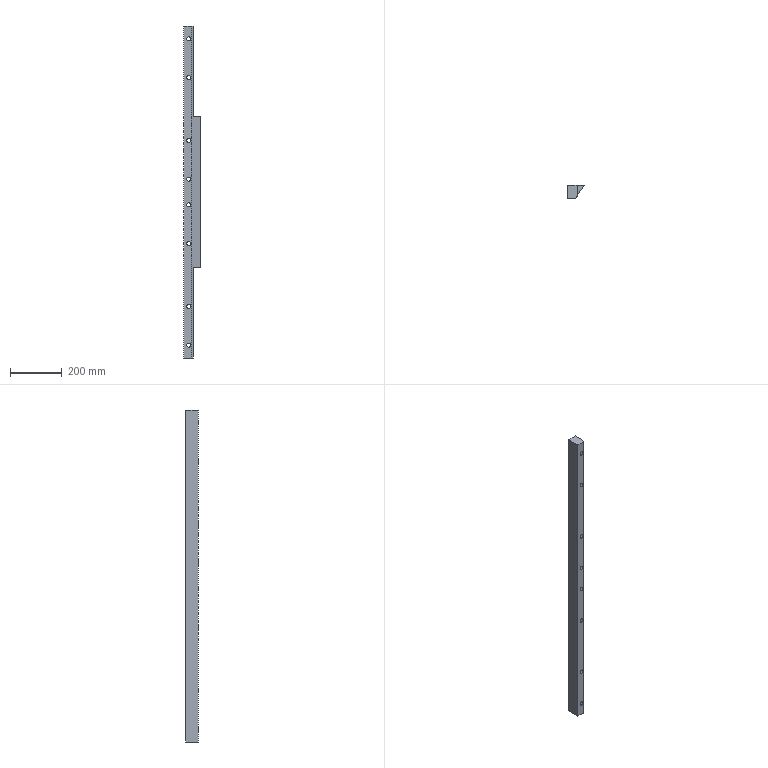Part | SolidWorks | features ICE 3, Extrusion 1, MirrorPattern 1 | 1 solid | 50 faces | box 64 x 50 x 1288 mm | volume 2493147 mm3 | cylinder 32 | plane 18 | commonest cylinder face diameters 16 x16 26 x16
STEP:
#1=CARTESIAN_POINT('',(20.,39.,1225.));
#2=VERTEX_POINT('',#1);
#3=CARTESIAN_POINT('',(20.,39.,1251.));
#4=VERTEX_POINT('',#3);
#5=CARTESIAN_POINT('',(20.,39.,1238.));
#6=DIRECTION('',(0.,1.,0.));
#7=DIRECTION('',(0.,0.,1.));
#8=AXIS2_PLACEMENT_3D('',#5,#6,#7);
#9=CIRCLE('',#8,13.);
#10=EDGE_CURVE('',#2,#4,#9,.T.);
#11=ORIENTED_EDGE('',*,*,#10,.F.);
#12=CARTESIAN_POINT('',(20.,50.,1225.));
#13=VERTEX_POINT('',#12);
#14=CARTESIAN_POINT('',(20.,39.,1225.));
#15=DIRECTION('',(0.,1.,0.));
#16=VECTOR('',#15,1000.);
#17=LINE('',#14,#16);
#18=EDGE_CURVE('',#2,#13,#17,.T.);
#19=ORIENTED_EDGE('',*,*,#18,.T.);
#20=CARTESIAN_POINT('',(20.,50.,1251.));
#21=VERTEX_POINT('',#20);
#22=CARTESIAN_POINT('',(20.,50.,1238.));
#23=DIRECTION('',(0.,1.,0.));
#24=DIRECTION('',(0.,0.,1.));
#25=AXIS2_PLACEMENT_3D('',#22,#23,#24);
#26=CIRCLE('',#25,13.);
#27=EDGE_CURVE('',#13,#21,#26,.T.);
#28=ORIENTED_EDGE('',*,*,#27,.T.);
#29=CARTESIAN_POINT('',(20.,39.,1251.));
#30=DIRECTION('',(0.,1.,0.));
#31=VECTOR('',#30,1000.);
#32=LINE('',#29,#31);
#33=EDGE_CURVE('',#4,#21,#32,.T.);
#34=ORIENTED_EDGE('',*,*,#33,.F.);
#35=EDGE_LOOP('',(#11,#19,#28,#34));
#36=FACE_OUTER_BOUND('',#35,.T.);
#37=CARTESIAN_POINT('',(20.,39.,1238.));
#38=DIRECTION('',(0.,1.,0.));
#39=DIRECTION('',(0.,0.,1.));
#40=AXIS2_PLACEMENT_3D('',#37,#38,#39);
#41=CYLINDRICAL_SURFACE('',#40,13.);
#42=ADVANCED_FACE('',(#36),#41,.F.);
#43=CARTESIAN_POINT('',(20.,39.,1075.));
#44=VERTEX_POINT('',#43);
#45=CARTESIAN_POINT('',(20.,39.,1101.));
#46=VERTEX_POINT('',#45);
#47=CARTESIAN_POINT('',(20.,39.,1088.));
#48=DIRECTION('',(0.,1.,0.));
#49=DIRECTION('',(0.,0.,1.));
#50=AXIS2_PLACEMENT_3D('',#47,#48,#49);
#51=CIRCLE('',#50,13.);
#52=EDGE_CURVE('',#44,#46,#51,.T.);
#53=ORIENTED_EDGE('',*,*,#52,.F.);
#54=CARTESIAN_POINT('',(20.,50.,1075.));
#55=VERTEX_POINT('',#54);
#56=CARTESIAN_POINT('',(20.,39.,1075.));
#57=DIRECTION('',(0.,1.,0.));
#58=VECTOR('',#57,1000.);
#59=LINE('',#56,#58);
#60=EDGE_CURVE('',#44,#55,#59,.T.);
#61=ORIENTED_EDGE('',*,*,#60,.T.);
#62=CARTESIAN_POINT('',(20.,50.,1101.));
#63=VERTEX_POINT('',#62);
#64=CARTESIAN_POINT('',(20.,50.,1088.));
#65=DIRECTION('',(0.,1.,0.));
#66=DIRECTION('',(0.,0.,1.));
#67=AXIS2_PLACEMENT_3D('',#64,#65,#66);
#68=CIRCLE('',#67,13.);
#69=EDGE_CURVE('',#55,#63,#68,.T.);
#70=ORIENTED_EDGE('',*,*,#69,.T.);
#71=CARTESIAN_POINT('',(20.,39.,1101.));
#72=DIRECTION('',(0.,1.,0.));
#73=VECTOR('',#72,1000.);
#74=LINE('',#71,#73);
#75=EDGE_CURVE('',#46,#63,#74,.T.);
#76=ORIENTED_EDGE('',*,*,#75,.F.);
#77=EDGE_LOOP('',(#53,#61,#70,#76));
#78=FACE_OUTER_BOUND('',#77,.T.);
#79=CARTESIAN_POINT('',(20.,39.,1088.));
#80=DIRECTION('',(0.,1.,0.));
#81=DIRECTION('',(0.,0.,1.));
#82=AXIS2_PLACEMENT_3D('',#79,#80,#81);
#83=CYLINDRICAL_SURFACE('',#82,13.);
#84=ADVANCED_FACE('',(#78),#83,.F.);
#85=CARTESIAN_POINT('',(20.,39.,831.));
#86=VERTEX_POINT('',#85);
#87=CARTESIAN_POINT('',(20.,39.,857.));
#88=VERTEX_POINT('',#87);
#89=CARTESIAN_POINT('',(20.,39.,844.));
#90=DIRECTION('',(0.,1.,0.));
#91=DIRECTION('',(0.,0.,1.));
#92=AXIS2_PLACEMENT_3D('',#89,#90,#91);
#93=CIRCLE('',#92,13.);
#94=EDGE_CURVE('',#86,#88,#93,.T.);
#95=ORIENTED_EDGE('',*,*,#94,.F.);
#96=CARTESIAN_POINT('',(20.,50.,831.));
#97=VERTEX_POINT('',#96);
#98=CARTESIAN_POINT('',(20.,39.,831.));
#99=DIRECTION('',(0.,1.,0.));
#100=VECTOR('',#99,1000.);
#101=LINE('',#98,#100);
#102=EDGE_CURVE('',#86,#97,#101,.T.);
#103=ORIENTED_EDGE('',*,*,#102,.T.);
#104=CARTESIAN_POINT('',(20.,50.,857.));
#105=VERTEX_POINT('',#104);
#106=CARTESIAN_POINT('',(20.,50.,844.));
#107=DIRECTION('',(0.,1.,0.));
#108=DIRECTION('',(0.,0.,1.));
#109=AXIS2_PLACEMENT_3D('',#106,#107,#108);
#110=CIRCLE('',#109,13.);
#111=EDGE_CURVE('',#97,#105,#110,.T.);
#112=ORIENTED_EDGE('',*,*,#111,.T.);
#113=CARTESIAN_POINT('',(20.,39.,857.));
#114=DIRECTION('',(0.,1.,0.));
#115=VECTOR('',#114,1000.);
#116=LINE('',#113,#115);
#117=EDGE_CURVE('',#88,#105,#116,.T.);
#118=ORIENTED_EDGE('',*,*,#117,.F.);
#119=EDGE_LOOP('',(#95,#103,#112,#118));
#120=FACE_OUTER_BOUND('',#119,.T.);
#121=CARTESIAN_POINT('',(20.,39.,844.));
#122=DIRECTION('',(0.,1.,0.));
#123=DIRECTION('',(0.,0.,1.));
#124=AXIS2_PLACEMENT_3D('',#121,#122,#123);
#125=CYLINDRICAL_SURFACE('',#124,13.);
#126=ADVANCED_FACE('',(#120),#125,.F.);
#127=CARTESIAN_POINT('',(20.,39.,681.));
#128=VERTEX_POINT('',#127);
#129=CARTESIAN_POINT('',(20.,39.,707.));
#130=VERTEX_POINT('',#129);
#131=CARTESIAN_POINT('',(20.,39.,694.));
#132=DIRECTION('',(0.,1.,0.));
#133=DIRECTION('',(0.,0.,1.));
#134=AXIS2_PLACEMENT_3D('',#131,#132,#133);
#135=CIRCLE('',#134,13.);
#136=EDGE_CURVE('',#128,#130,#135,.T.);
#137=ORIENTED_EDGE('',*,*,#136,.F.);
#138=CARTESIAN_POINT('',(20.,50.,681.));
#139=VERTEX_POINT('',#138);
#140=CARTESIAN_POINT('',(20.,39.,681.));
#141=DIRECTION('',(0.,1.,0.));
#142=VECTOR('',#141,1000.);
#143=LINE('',#140,#142);
#144=EDGE_CURVE('',#128,#139,#143,.T.);
#145=ORIENTED_EDGE('',*,*,#144,.T.);
#146=CARTESIAN_POINT('',(20.,50.,707.));
#147=VERTEX_POINT('',#146);
#148=CARTESIAN_POINT('',(20.,50.,694.));
#149=DIRECTION('',(0.,1.,0.));
#150=DIRECTION('',(0.,0.,1.));
#151=AXIS2_PLACEMENT_3D('',#148,#149,#150);
#152=CIRCLE('',#151,13.);
#153=EDGE_CURVE('',#139,#147,#152,.T.);
#154=ORIENTED_EDGE('',*,*,#153,.T.);
#155=CARTESIAN_POINT('',(20.,39.,707.));
#156=DIRECTION('',(0.,1.,0.));
#157=VECTOR('',#156,1000.);
#158=LINE('',#155,#157);
#159=EDGE_CURVE('',#130,#147,#158,.T.);
#160=ORIENTED_EDGE('',*,*,#159,.F.);
#161=EDGE_LOOP('',(#137,#145,#154,#160));
#162=FACE_OUTER_BOUND('',#161,.T.);
#163=CARTESIAN_POINT('',(20.,39.,694.));
#164=DIRECTION('',(0.,1.,0.));
#165=DIRECTION('',(0.,0.,1.));
#166=AXIS2_PLACEMENT_3D('',#163,#164,#165);
#167=CYLINDRICAL_SURFACE('',#166,13.);
#168=ADVANCED_FACE('',(#162),#167,.F.);
#169=CARTESIAN_POINT('',(20.,39.,581.));
#170=VERTEX_POINT('',#169);
#171=CARTESIAN_POINT('',(20.,39.,607.));
#172=VERTEX_POINT('',#171);
#173=CARTESIAN_POINT('',(20.,39.,594.));
#174=DIRECTION('',(0.,1.,0.));
#175=DIRECTION('',(0.,0.,1.));
#176=AXIS2_PLACEMENT_3D('',#173,#174,#175);
#177=CIRCLE('',#176,13.);
#178=EDGE_CURVE('',#170,#172,#177,.T.);
#179=ORIENTED_EDGE('',*,*,#178,.F.);
#180=CARTESIAN_POINT('',(20.,50.,581.));
#181=VERTEX_POINT('',#180);
#182=CARTESIAN_POINT('',(20.,39.,581.));
#183=DIRECTION('',(0.,1.,0.));
#184=VECTOR('',#183,1000.);
#185=LINE('',#182,#184);
#186=EDGE_CURVE('',#170,#181,#185,.T.);
#187=ORIENTED_EDGE('',*,*,#186,.T.);
#188=CARTESIAN_POINT('',(20.,50.,607.));
#189=VERTEX_POINT('',#188);
#190=CARTESIAN_POINT('',(20.,50.,594.));
#191=DIRECTION('',(0.,1.,0.));
#192=DIRECTION('',(0.,0.,1.));
#193=AXIS2_PLACEMENT_3D('',#190,#191,#192);
#194=CIRCLE('',#193,13.);
#195=EDGE_CURVE('',#181,#189,#194,.T.);
#196=ORIENTED_EDGE('',*,*,#195,.T.);
#197=CARTESIAN_POINT('',(20.,39.,607.));
#198=DIRECTION('',(0.,1.,0.));
#199=VECTOR('',#198,1000.);
#200=LINE('',#197,#199);
#201=EDGE_CURVE('',#172,#189,#200,.T.);
#202=ORIENTED_EDGE('',*,*,#201,.F.);
#203=EDGE_LOOP('',(#179,#187,#196,#202));
#204=FACE_OUTER_BOUND('',#203,.T.);
#205=CARTESIAN_POINT('',(20.,39.,594.));
#206=DIRECTION('',(0.,1.,0.));
#207=DIRECTION('',(0.,0.,1.));
#208=AXIS2_PLACEMENT_3D('',#205,#206,#207);
#209=CYLINDRICAL_SURFACE('',#208,13.);
#210=ADVANCED_FACE('',(#204),#209,.F.);
#211=CARTESIAN_POINT('',(20.,39.,431.));
#212=VERTEX_POINT('',#211);
#213=CARTESIAN_POINT('',(20.,39.,457.));
#214=VERTEX_POINT('',#213);
#215=CARTESIAN_POINT('',(20.,39.,444.));
#216=DIRECTION('',(0.,1.,0.));
#217=DIRECTION('',(0.,0.,1.));
#218=AXIS2_PLACEMENT_3D('',#215,#216,#217);
#219=CIRCLE('',#218,13.);
#220=EDGE_CURVE('',#212,#214,#219,.T.);
#221=ORIENTED_EDGE('',*,*,#220,.F.);
#222=CARTESIAN_POINT('',(20.,50.,431.));
#223=VERTEX_POINT('',#222);
#224=CARTESIAN_POINT('',(20.,39.,431.));
#225=DIRECTION('',(0.,1.,0.));
#226=VECTOR('',#225,1000.);
#227=LINE('',#224,#226);
#228=EDGE_CURVE('',#212,#223,#227,.T.);
#229=ORIENTED_EDGE('',*,*,#228,.T.);
#230=CARTESIAN_POINT('',(20.,50.,457.));
#231=VERTEX_POINT('',#230);
#232=CARTESIAN_POINT('',(20.,50.,444.));
#233=DIRECTION('',(0.,1.,0.));
#234=DIRECTION('',(0.,0.,1.));
#235=AXIS2_PLACEMENT_3D('',#232,#233,#234);
#236=CIRCLE('',#235,13.);
#237=EDGE_CURVE('',#223,#231,#236,.T.);
#238=ORIENTED_EDGE('',*,*,#237,.T.);
#239=CARTESIAN_POINT('',(20.,39.,457.));
#240=DIRECTION('',(0.,1.,0.));
#241=VECTOR('',#240,1000.);
#242=LINE('',#239,#241);
#243=EDGE_CURVE('',#214,#231,#242,.T.);
#244=ORIENTED_EDGE('',*,*,#243,.F.);
#245=EDGE_LOOP('',(#221,#229,#238,#244));
#246=FACE_OUTER_BOUND('',#245,.T.);
#247=CARTESIAN_POINT('',(20.,39.,444.));
#248=DIRECTION('',(0.,1.,0.));
#249=DIRECTION('',(0.,0.,1.));
#250=AXIS2_PLACEMENT_3D('',#247,#248,#249);
#251=CYLINDRICAL_SURFACE('',#250,13.);
#252=ADVANCED_FACE('',(#246),#251,.F.);
#253=CARTESIAN_POINT('',(20.,39.,187.));
#254=VERTEX_POINT('',#253);
#255=CARTESIAN_POINT('',(20.,39.,213.));
#256=VERTEX_POINT('',#255);
#257=CARTESIAN_POINT('',(20.,39.,200.));
#258=DIRECTION('',(0.,1.,0.));
#259=DIRECTION('',(0.,0.,1.));
#260=AXIS2_PLACEMENT_3D('',#257,#258,#259);
#261=CIRCLE('',#260,13.);
#262=EDGE_CURVE('',#254,#256,#261,.T.);
#263=ORIENTED_EDGE('',*,*,#262,.F.);
#264=CARTESIAN_POINT('',(20.,50.,187.));
#265=VERTEX_POINT('',#264);
#266=CARTESIAN_POINT('',(20.,39.,187.));
#267=DIRECTION('',(0.,1.,0.));
#268=VECTOR('',#267,1000.);
#269=LINE('',#266,#268);
#270=EDGE_CURVE('',#254,#265,#269,.T.);
#271=ORIENTED_EDGE('',*,*,#270,.T.);
#272=CARTESIAN_POINT('',(20.,50.,213.));
#273=VERTEX_POINT('',#272);
#274=CARTESIAN_POINT('',(20.,50.,200.));
#275=DIRECTION('',(0.,1.,0.));
#276=DIRECTION('',(0.,0.,1.));
#277=AXIS2_PLACEMENT_3D('',#274,#275,#276);
#278=CIRCLE('',#277,13.);
#279=EDGE_CURVE('',#265,#273,#278,.T.);
#280=ORIENTED_EDGE('',*,*,#279,.T.);
#281=CARTESIAN_POINT('',(20.,39.,213.));
#282=DIRECTION('',(0.,1.,0.));
#283=VECTOR('',#282,1000.);
#284=LINE('',#281,#283);
#285=EDGE_CURVE('',#256,#273,#284,.T.);
#286=ORIENTED_EDGE('',*,*,#285,.F.);
#287=EDGE_LOOP('',(#263,#271,#280,#286));
#288=FACE_OUTER_BOUND('',#287,.T.);
#289=CARTESIAN_POINT('',(20.,39.,200.));
#290=DIRECTION('',(0.,1.,0.));
#291=DIRECTION('',(0.,0.,1.));
#292=AXIS2_PLACEMENT_3D('',#289,#290,#291);
#293=CYLINDRICAL_SURFACE('',#292,13.);
#294=ADVANCED_FACE('',(#288),#293,.F.);
#295=CARTESIAN_POINT('',(20.,39.,37.));
#296=VERTEX_POINT('',#295);
#297=CARTESIAN_POINT('',(20.,39.,63.));
#298=VERTEX_POINT('',#297);
#299=CARTESIAN_POINT('',(20.,39.,50.));
#300=DIRECTION('',(0.,1.,0.));
#301=DIRECTION('',(0.,0.,1.));
#302=AXIS2_PLACEMENT_3D('',#299,#300,#301);
#303=CIRCLE('',#302,13.);
#304=EDGE_CURVE('',#296,#298,#303,.T.);
#305=ORIENTED_EDGE('',*,*,#304,.F.);
#306=CARTESIAN_POINT('',(20.,50.,37.));
#307=VERTEX_POINT('',#306);
#308=CARTESIAN_POINT('',(20.,39.,37.));
#309=DIRECTION('',(0.,1.,0.));
#310=VECTOR('',#309,1000.);
#311=LINE('',#308,#310);
#312=EDGE_CURVE('',#296,#307,#311,.T.);
#313=ORIENTED_EDGE('',*,*,#312,.T.);
#314=CARTESIAN_POINT('',(20.,50.,63.));
#315=VERTEX_POINT('',#314);
#316=CARTESIAN_POINT('',(20.,50.,50.));
#317=DIRECTION('',(0.,1.,0.));
#318=DIRECTION('',(0.,0.,1.));
#319=AXIS2_PLACEMENT_3D('',#316,#317,#318);
#320=CIRCLE('',#319,13.);
#321=EDGE_CURVE('',#307,#315,#320,.T.);
#322=ORIENTED_EDGE('',*,*,#321,.T.);
#323=CARTESIAN_POINT('',(20.,39.,63.));
#324=DIRECTION('',(0.,1.,0.));
#325=VECTOR('',#324,1000.);
#326=LINE('',#323,#325);
#327=EDGE_CURVE('',#298,#315,#326,.T.);
#328=ORIENTED_EDGE('',*,*,#327,.F.);
#329=EDGE_LOOP('',(#305,#313,#322,#328));
#330=FACE_OUTER_BOUND('',#329,.T.);
#331=CARTESIAN_POINT('',(20.,39.,50.));
#332=DIRECTION('',(0.,1.,0.));
#333=DIRECTION('',(0.,0.,1.));
#334=AXIS2_PLACEMENT_3D('',#331,#332,#333);
#335=CYLINDRICAL_SURFACE('',#334,13.);
#336=ADVANCED_FACE('',(#330),#335,.F.);
#337=CARTESIAN_POINT('',(20.,0.,42.));
#338=VERTEX_POINT('',#337);
#339=CARTESIAN_POINT('',(20.,0.,58.));
#340=VERTEX_POINT('',#339);
#341=CARTESIAN_POINT('',(20.,0.,50.));
#342=DIRECTION('',(0.,1.,0.));
#343=DIRECTION('',(0.,0.,1.));
#344=AXIS2_PLACEMENT_3D('',#341,#342,#343);
#345=CIRCLE('',#344,8.);
#346=EDGE_CURVE('',#338,#340,#345,.T.);
#347=ORIENTED_EDGE('',*,*,#346,.F.);
#348=CARTESIAN_POINT('',(20.,39.,42.));
#349=VERTEX_POINT('',#348);
#350=CARTESIAN_POINT('',(20.,-675.,42.));
#351=DIRECTION('',(0.,1.,0.));
#352=VECTOR('',#351,1000.);
#353=LINE('',#350,#352);
#354=EDGE_CURVE('',#338,#349,#353,.T.);
#355=ORIENTED_EDGE('',*,*,#354,.T.);
#356=CARTESIAN_POINT('',(20.,39.,58.));
#357=VERTEX_POINT('',#356);
#358=CARTESIAN_POINT('',(20.,39.,50.));
#359=DIRECTION('',(0.,-1.,0.));
#360=DIRECTION('',(0.,0.,1.));
#361=AXIS2_PLACEMENT_3D('',#358,#359,#360);
#362=CIRCLE('',#361,8.);
#363=EDGE_CURVE('',#357,#349,#362,.T.);
#364=ORIENTED_EDGE('',*,*,#363,.F.);
#365=CARTESIAN_POINT('',(20.,-675.,58.));
#366=DIRECTION('',(0.,1.,0.));
#367=VECTOR('',#366,1000.);
#368=LINE('',#365,#367);
#369=EDGE_CURVE('',#340,#357,#368,.T.);
#370=ORIENTED_EDGE('',*,*,#369,.F.);
#371=EDGE_LOOP('',(#347,#355,#364,#370));
#372=FACE_OUTER_BOUND('',#371,.T.);
#373=CARTESIAN_POINT('',(20.,-675.,50.));
#374=DIRECTION('',(0.,1.,0.));
#375=DIRECTION('',(0.,0.,1.));
#376=AXIS2_PLACEMENT_3D('',#373,#374,#375);
#377=CYLINDRICAL_SURFACE('',#376,8.);
#378=ADVANCED_FACE('',(#372),#377,.F.);
#379=CARTESIAN_POINT('',(20.,0.,192.));
#380=VERTEX_POINT('',#379);
#381=CARTESIAN_POINT('',(20.,0.,208.));
#382=VERTEX_POINT('',#381);
#383=CARTESIAN_POINT('',(20.,0.,200.));
#384=DIRECTION('',(0.,1.,0.));
#385=DIRECTION('',(0.,0.,1.));
#386=AXIS2_PLACEMENT_3D('',#383,#384,#385);
#387=CIRCLE('',#386,8.);
#388=EDGE_CURVE('',#380,#382,#387,.T.);
#389=ORIENTED_EDGE('',*,*,#388,.F.);
#390=CARTESIAN_POINT('',(20.,39.,192.));
#391=VERTEX_POINT('',#390);
#392=CARTESIAN_POINT('',(20.,-675.,192.));
#393=DIRECTION('',(0.,1.,0.));
#394=VECTOR('',#393,1000.);
#395=LINE('',#392,#394);
#396=EDGE_CURVE('',#380,#391,#395,.T.);
#397=ORIENTED_EDGE('',*,*,#396,.T.);
#398=CARTESIAN_POINT('',(20.,39.,208.));
#399=VERTEX_POINT('',#398);
#400=CARTESIAN_POINT('',(20.,39.,200.));
#401=DIRECTION('',(0.,-1.,0.));
#402=DIRECTION('',(0.,0.,1.));
#403=AXIS2_PLACEMENT_3D('',#400,#401,#402);
#404=CIRCLE('',#403,8.);
#405=EDGE_CURVE('',#399,#391,#404,.T.);
#406=ORIENTED_EDGE('',*,*,#405,.F.);
#407=CARTESIAN_POINT('',(20.,-675.,208.));
#408=DIRECTION('',(0.,1.,0.));
#409=VECTOR('',#408,1000.);
#410=LINE('',#407,#409);
#411=EDGE_CURVE('',#382,#399,#410,.T.);
#412=ORIENTED_EDGE('',*,*,#411,.F.);
#413=EDGE_LOOP('',(#389,#397,#406,#412));
#414=FACE_OUTER_BOUND('',#413,.T.);
#415=CARTESIAN_POINT('',(20.,-675.,200.));
#416=DIRECTION('',(0.,1.,0.));
#417=DIRECTION('',(0.,0.,1.));
#418=AXIS2_PLACEMENT_3D('',#415,#416,#417);
#419=CYLINDRICAL_SURFACE('',#418,8.);
#420=ADVANCED_FACE('',(#414),#419,.F.);
#421=CARTESIAN_POINT('',(20.,0.,436.));
#422=VERTEX_POINT('',#421);
#423=CARTESIAN_POINT('',(20.,0.,452.));
#424=VERTEX_POINT('',#423);
#425=CARTESIAN_POINT('',(20.,0.,444.));
#426=DIRECTION('',(0.,1.,0.));
#427=DIRECTION('',(0.,0.,1.));
#428=AXIS2_PLACEMENT_3D('',#425,#426,#427);
#429=CIRCLE('',#428,8.);
#430=EDGE_CURVE('',#422,#424,#429,.T.);
#431=ORIENTED_EDGE('',*,*,#430,.F.);
#432=CARTESIAN_POINT('',(20.,39.,436.));
#433=VERTEX_POINT('',#432);
#434=CARTESIAN_POINT('',(20.,-675.,436.));
#435=DIRECTION('',(0.,1.,0.));
#436=VECTOR('',#435,1000.);
#437=LINE('',#434,#436);
#438=EDGE_CURVE('',#422,#433,#437,.T.);
#439=ORIENTED_EDGE('',*,*,#438,.T.);
#440=CARTESIAN_POINT('',(20.,39.,452.));
#441=VERTEX_POINT('',#440);
#442=CARTESIAN_POINT('',(20.,39.,444.));
#443=DIRECTION('',(0.,-1.,0.));
#444=DIRECTION('',(0.,0.,1.));
#445=AXIS2_PLACEMENT_3D('',#442,#443,#444);
#446=CIRCLE('',#445,8.);
#447=EDGE_CURVE('',#441,#433,#446,.T.);
#448=ORIENTED_EDGE('',*,*,#447,.F.);
#449=CARTESIAN_POINT('',(20.,-675.,452.));
#450=DIRECTION('',(0.,1.,0.));
#451=VECTOR('',#450,1000.);
#452=LINE('',#449,#451);
#453=EDGE_CURVE('',#424,#441,#452,.T.);
#454=ORIENTED_EDGE('',*,*,#453,.F.);
#455=EDGE_LOOP('',(#431,#439,#448,#454));
#456=FACE_OUTER_BOUND('',#455,.T.);
#457=CARTESIAN_POINT('',(20.,-675.,444.));
#458=DIRECTION('',(0.,1.,0.));
#459=DIRECTION('',(0.,0.,1.));
#460=AXIS2_PLACEMENT_3D('',#457,#458,#459);
#461=CYLINDRICAL_SURFACE('',#460,8.);
#462=ADVANCED_FACE('',(#456),#461,.F.);
#463=CARTESIAN_POINT('',(20.,0.,586.));
#464=VERTEX_POINT('',#463);
#465=CARTESIAN_POINT('',(20.,0.,602.));
#466=VERTEX_POINT('',#465);
#467=CARTESIAN_POINT('',(20.,0.,594.));
#468=DIRECTION('',(0.,1.,0.));
#469=DIRECTION('',(0.,0.,1.));
#470=AXIS2_PLACEMENT_3D('',#467,#468,#469);
#471=CIRCLE('',#470,8.);
#472=EDGE_CURVE('',#464,#466,#471,.T.);
#473=ORIENTED_EDGE('',*,*,#472,.F.);
#474=CARTESIAN_POINT('',(20.,39.,586.));
#475=VERTEX_POINT('',#474);
#476=CARTESIAN_POINT('',(20.,-675.,586.));
#477=DIRECTION('',(0.,1.,0.));
#478=VECTOR('',#477,1000.);
#479=LINE('',#476,#478);
#480=EDGE_CURVE('',#464,#475,#479,.T.);
#481=ORIENTED_EDGE('',*,*,#480,.T.);
#482=CARTESIAN_POINT('',(20.,39.,602.));
#483=VERTEX_POINT('',#482);
#484=CARTESIAN_POINT('',(20.,39.,594.));
#485=DIRECTION('',(0.,-1.,0.));
#486=DIRECTION('',(0.,0.,1.));
#487=AXIS2_PLACEMENT_3D('',#484,#485,#486);
#488=CIRCLE('',#487,8.);
#489=EDGE_CURVE('',#483,#475,#488,.T.);
#490=ORIENTED_EDGE('',*,*,#489,.F.);
#491=CARTESIAN_POINT('',(20.,-675.,602.));
#492=DIRECTION('',(0.,1.,0.));
#493=VECTOR('',#492,1000.);
#494=LINE('',#491,#493);
#495=EDGE_CURVE('',#466,#483,#494,.T.);
#496=ORIENTED_EDGE('',*,*,#495,.F.);
#497=EDGE_LOOP('',(#473,#481,#490,#496));
#498=FACE_OUTER_BOUND('',#497,.T.);
#499=CARTESIAN_POINT('',(20.,-675.,594.));
#500=DIRECTION('',(0.,1.,0.));
#501=DIRECTION('',(0.,0.,1.));
#502=AXIS2_PLACEMENT_3D('',#499,#500,#501);
#503=CYLINDRICAL_SURFACE('',#502,8.);
#504=ADVANCED_FACE('',(#498),#503,.F.);
#505=CARTESIAN_POINT('',(20.,0.,686.));
#506=VERTEX_POINT('',#505);
#507=CARTESIAN_POINT('',(20.,0.,702.));
#508=VERTEX_POINT('',#507);
#509=CARTESIAN_POINT('',(20.,0.,694.));
#510=DIRECTION('',(0.,1.,0.));
#511=DIRECTION('',(0.,0.,1.));
#512=AXIS2_PLACEMENT_3D('',#509,#510,#511);
#513=CIRCLE('',#512,8.);
#514=EDGE_CURVE('',#506,#508,#513,.T.);
#515=ORIENTED_EDGE('',*,*,#514,.F.);
#516=CARTESIAN_POINT('',(20.,39.,686.));
#517=VERTEX_POINT('',#516);
#518=CARTESIAN_POINT('',(20.,-675.,686.));
#519=DIRECTION('',(0.,1.,0.));
#520=VECTOR('',#519,1000.);
#521=LINE('',#518,#520);
#522=EDGE_CURVE('',#506,#517,#521,.T.);
#523=ORIENTED_EDGE('',*,*,#522,.T.);
#524=CARTESIAN_POINT('',(20.,39.,702.));
#525=VERTEX_POINT('',#524);
#526=CARTESIAN_POINT('',(20.,39.,694.));
#527=DIRECTION('',(0.,-1.,0.));
#528=DIRECTION('',(0.,0.,1.));
#529=AXIS2_PLACEMENT_3D('',#526,#527,#528);
#530=CIRCLE('',#529,8.);
#531=EDGE_CURVE('',#525,#517,#530,.T.);
#532=ORIENTED_EDGE('',*,*,#531,.F.);
#533=CARTESIAN_POINT('',(20.,-675.,702.));
#534=DIRECTION('',(0.,1.,0.));
#535=VECTOR('',#534,1000.);
#536=LINE('',#533,#535);
#537=EDGE_CURVE('',#508,#525,#536,.T.);
#538=ORIENTED_EDGE('',*,*,#537,.F.);
#539=EDGE_LOOP('',(#515,#523,#532,#538));
#540=FACE_OUTER_BOUND('',#539,.T.);
#541=CARTESIAN_POINT('',(20.,-675.,694.));
#542=DIRECTION('',(0.,1.,0.));
#543=DIRECTION('',(0.,0.,1.));
#544=AXIS2_PLACEMENT_3D('',#541,#542,#543);
#545=CYLINDRICAL_SURFACE('',#544,8.);
#546=ADVANCED_FACE('',(#540),#545,.F.);
#547=CARTESIAN_POINT('',(20.,0.,836.));
#548=VERTEX_POINT('',#547);
#549=CARTESIAN_POINT('',(20.,0.,852.));
#550=VERTEX_POINT('',#549);
#551=CARTESIAN_POINT('',(20.,0.,844.));
#552=DIRECTION('',(0.,1.,0.));
#553=DIRECTION('',(0.,0.,1.));
#554=AXIS2_PLACEMENT_3D('',#551,#552,#553);
#555=CIRCLE('',#554,8.);
#556=EDGE_CURVE('',#548,#550,#555,.T.);
#557=ORIENTED_EDGE('',*,*,#556,.F.);
#558=CARTESIAN_POINT('',(20.,39.,836.));
#559=VERTEX_POINT('',#558);
#560=CARTESIAN_POINT('',(20.,-675.,836.));
#561=DIRECTION('',(0.,1.,0.));
#562=VECTOR('',#561,1000.);
#563=LINE('',#560,#562);
#564=EDGE_CURVE('',#548,#559,#563,.T.);
#565=ORIENTED_EDGE('',*,*,#564,.T.);
#566=CARTESIAN_POINT('',(20.,39.,852.));
#567=VERTEX_POINT('',#566);
#568=CARTESIAN_POINT('',(20.,39.,844.));
#569=DIRECTION('',(0.,-1.,0.));
#570=DIRECTION('',(0.,0.,1.));
#571=AXIS2_PLACEMENT_3D('',#568,#569,#570);
#572=CIRCLE('',#571,8.);
#573=EDGE_CURVE('',#567,#559,#572,.T.);
#574=ORIENTED_EDGE('',*,*,#573,.F.);
#575=CARTESIAN_POINT('',(20.,-675.,852.));
#576=DIRECTION('',(0.,1.,0.));
#577=VECTOR('',#576,1000.);
#578=LINE('',#575,#577);
#579=EDGE_CURVE('',#550,#567,#578,.T.);
#580=ORIENTED_EDGE('',*,*,#579,.F.);
#581=EDGE_LOOP('',(#557,#565,#574,#580));
#582=FACE_OUTER_BOUND('',#581,.T.);
#583=CARTESIAN_POINT('',(20.,-675.,844.));
#584=DIRECTION('',(0.,1.,0.));
#585=DIRECTION('',(0.,0.,1.));
#586=AXIS2_PLACEMENT_3D('',#583,#584,#585);
#587=CYLINDRICAL_SURFACE('',#586,8.);
#588=ADVANCED_FACE('',(#582),#587,.F.);
#589=CARTESIAN_POINT('',(20.,0.,1080.));
#590=VERTEX_POINT('',#589);
#591=CARTESIAN_POINT('',(20.,0.,1096.));
#592=VERTEX_POINT('',#591);
#593=CARTESIAN_POINT('',(20.,0.,1088.));
#594=DIRECTION('',(0.,1.,0.));
#595=DIRECTION('',(0.,0.,1.));
#596=AXIS2_PLACEMENT_3D('',#593,#594,#595);
#597=CIRCLE('',#596,8.);
#598=EDGE_CURVE('',#590,#592,#597,.T.);
#599=ORIENTED_EDGE('',*,*,#598,.F.);
#600=CARTESIAN_POINT('',(20.,39.,1080.));
#601=VERTEX_POINT('',#600);
#602=CARTESIAN_POINT('',(20.,-675.,1080.));
#603=DIRECTION('',(0.,1.,0.));
#604=VECTOR('',#603,1000.);
#605=LINE('',#602,#604);
#606=EDGE_CURVE('',#590,#601,#605,.T.);
#607=ORIENTED_EDGE('',*,*,#606,.T.);
#608=CARTESIAN_POINT('',(20.,39.,1096.));
#609=VERTEX_POINT('',#608);
#610=CARTESIAN_POINT('',(20.,39.,1088.));
#611=DIRECTION('',(0.,-1.,0.));
#612=DIRECTION('',(0.,0.,1.));
#613=AXIS2_PLACEMENT_3D('',#610,#611,#612);
#614=CIRCLE('',#613,8.);
#615=EDGE_CURVE('',#609,#601,#614,.T.);
#616=ORIENTED_EDGE('',*,*,#615,.F.);
#617=CARTESIAN_POINT('',(20.,-675.,1096.));
#618=DIRECTION('',(0.,1.,0.));
#619=VECTOR('',#618,1000.);
#620=LINE('',#617,#619);
#621=EDGE_CURVE('',#592,#609,#620,.T.);
#622=ORIENTED_EDGE('',*,*,#621,.F.);
#623=EDGE_LOOP('',(#599,#607,#616,#622));
#624=FACE_OUTER_BOUND('',#623,.T.);
#625=CARTESIAN_POINT('',(20.,-675.,1088.));
#626=DIRECTION('',(0.,1.,0.));
#627=DIRECTION('',(0.,0.,1.));
#628=AXIS2_PLACEMENT_3D('',#625,#626,#627);
#629=CYLINDRICAL_SURFACE('',#628,8.);
#630=ADVANCED_FACE('',(#624),#629,.F.);
#631=CARTESIAN_POINT('',(20.,0.,1230.));
#632=VERTEX_POINT('',#631);
#633=CARTESIAN_POINT('',(20.,0.,1246.));
#634=VERTEX_POINT('',#633);
#635=CARTESIAN_POINT('',(20.,0.,1238.));
#636=DIRECTION('',(0.,1.,0.));
#637=DIRECTION('',(0.,0.,1.));
#638=AXIS2_PLACEMENT_3D('',#635,#636,#637);
#639=CIRCLE('',#638,8.);
#640=EDGE_CURVE('',#632,#634,#639,.T.);
#641=ORIENTED_EDGE('',*,*,#640,.F.);
#642=CARTESIAN_POINT('',(20.,39.,1230.));
#643=VERTEX_POINT('',#642);
#644=CARTESIAN_POINT('',(20.,-675.,1230.));
#645=DIRECTION('',(0.,1.,0.));
#646=VECTOR('',#645,1000.);
#647=LINE('',#644,#646);
#648=EDGE_CURVE('',#632,#643,#647,.T.);
#649=ORIENTED_EDGE('',*,*,#648,.T.);
#650=CARTESIAN_POINT('',(20.,39.,1246.));
#651=VERTEX_POINT('',#650);
#652=CARTESIAN_POINT('',(20.,39.,1238.));
#653=DIRECTION('',(0.,-1.,0.));
#654=DIRECTION('',(0.,0.,1.));
#655=AXIS2_PLACEMENT_3D('',#652,#653,#654);
#656=CIRCLE('',#655,8.);
#657=EDGE_CURVE('',#651,#643,#656,.T.);
#658=ORIENTED_EDGE('',*,*,#657,.F.);
#659=CARTESIAN_POINT('',(20.,-675.,1246.));
#660=DIRECTION('',(0.,1.,0.));
#661=VECTOR('',#660,1000.);
#662=LINE('',#659,#661);
#663=EDGE_CURVE('',#634,#651,#662,.T.);
#664=ORIENTED_EDGE('',*,*,#663,.F.);
#665=EDGE_LOOP('',(#641,#649,#658,#664));
#666=FACE_OUTER_BOUND('',#665,.T.);
#667=CARTESIAN_POINT('',(20.,-675.,1238.));
#668=DIRECTION('',(0.,1.,0.));
#669=DIRECTION('',(0.,0.,1.));
#670=AXIS2_PLACEMENT_3D('',#667,#668,#669);
#671=CYLINDRICAL_SURFACE('',#670,8.);
#672=ADVANCED_FACE('',(#666),#671,.F.);
#673=CARTESIAN_POINT('',(36.,10.,350.));
#674=VERTEX_POINT('',#673);
#675=CARTESIAN_POINT('',(36.,10.,0.));
#676=VERTEX_POINT('',#675);
#677=CARTESIAN_POINT('',(36.,10.,350.));
#678=DIRECTION('',(0.,0.,-1.));
#679=VECTOR('',#678,1000.);
#680=LINE('',#677,#679);
#681=EDGE_CURVE('',#674,#676,#680,.T.);
#682=ORIENTED_EDGE('',*,*,#681,.F.);
#683=CARTESIAN_POINT('',(64.,50.,350.));
#684=VERTEX_POINT('',#683);
#685=CARTESIAN_POINT('',(36.,10.,350.));
#686=DIRECTION('',(0.5735,0.8192,0.));
#687=VECTOR('',#686,1000.);
#688=LINE('',#685,#687);
#689=EDGE_CURVE('',#674,#684,#688,.T.);
#690=ORIENTED_EDGE('',*,*,#689,.T.);
#691=CARTESIAN_POINT('',(64.,50.,938.));
#692=VERTEX_POINT('',#691);
#693=CARTESIAN_POINT('',(64.,50.,1288.));
#694=DIRECTION('',(0.,0.,-1.));
#695=VECTOR('',#694,1000.);
#696=LINE('',#693,#695);
#697=EDGE_CURVE('',#692,#684,#696,.T.);
#698=ORIENTED_EDGE('',*,*,#697,.F.);
#699=CARTESIAN_POINT('',(36.,10.,938.));
#700=VERTEX_POINT('',#699);
#701=CARTESIAN_POINT('',(36.,10.,938.));
#702=DIRECTION('',(0.5735,0.8192,0.));
#703=VECTOR('',#702,1000.);
#704=LINE('',#701,#703);
#705=EDGE_CURVE('',#700,#692,#704,.T.);
#706=ORIENTED_EDGE('',*,*,#705,.F.);
#707=CARTESIAN_POINT('',(36.,10.,1288.));
#708=VERTEX_POINT('',#707);
#709=CARTESIAN_POINT('',(36.,10.,938.));
#710=DIRECTION('',(0.,0.,1.));
#711=VECTOR('',#710,1000.);
#712=LINE('',#709,#711);
#713=EDGE_CURVE('',#700,#708,#712,.T.);
#714=ORIENTED_EDGE('',*,*,#713,.T.);
#715=CARTESIAN_POINT('',(29.,0.,1288.));
#716=VERTEX_POINT('',#715);
#717=CARTESIAN_POINT('',(64.,50.,1288.));
#718=DIRECTION('',(0.5735,0.8192,0.));
#719=VECTOR('',#718,1000.);
#720=LINE('',#717,#719);
#721=EDGE_CURVE('',#716,#708,#720,.T.);
#722=ORIENTED_EDGE('',*,*,#721,.F.);
#723=CARTESIAN_POINT('',(29.,0.,0.));
#724=VERTEX_POINT('',#723);
#725=CARTESIAN_POINT('',(29.,0.,1288.));
#726=DIRECTION('',(0.,0.,-1.));
#727=VECTOR('',#726,1000.);
#728=LINE('',#725,#727);
#729=EDGE_CURVE('',#716,#724,#728,.T.);
#730=ORIENTED_EDGE('',*,*,#729,.T.);
#731=CARTESIAN_POINT('',(64.,50.,0.));
#732=DIRECTION('',(0.5735,0.8192,0.));
#733=VECTOR('',#732,1000.);
#734=LINE('',#731,#733);
#735=EDGE_CURVE('',#724,#676,#734,.T.);
#736=ORIENTED_EDGE('',*,*,#735,.T.);
#737=EDGE_LOOP('',(#682,#690,#698,#706,#714,#722,#730,#736));
#738=FACE_OUTER_BOUND('',#737,.T.);
#739=CARTESIAN_POINT('',(64.,50.,1288.));
#740=DIRECTION('',(-0.8192,0.5735,0.));
#741=DIRECTION('',(-0.5735,-0.8192,0.));
#742=AXIS2_PLACEMENT_3D('',#739,#740,#741);
#743=PLANE('',#742);
#744=ADVANCED_FACE('',(#738),#743,.F.);
#745=CARTESIAN_POINT('',(20.,50.,50.));
#746=DIRECTION('',(0.,1.,0.));
#747=DIRECTION('',(0.,0.,1.));
#748=AXIS2_PLACEMENT_3D('',#745,#746,#747);
#749=CIRCLE('',#748,13.);
#750=EDGE_CURVE('',#315,#307,#749,.T.);
#751=ORIENTED_EDGE('',*,*,#750,.F.);
#752=ORIENTED_EDGE('',*,*,#321,.F.);
#753=EDGE_LOOP('',(#751,#752));
#754=FACE_BOUND('',#753,.T.);
#755=CARTESIAN_POINT('',(20.,50.,1238.));
#756=DIRECTION('',(0.,1.,0.));
#757=DIRECTION('',(0.,0.,1.));
#758=AXIS2_PLACEMENT_3D('',#755,#756,#757);
#759=CIRCLE('',#758,13.);
#760=EDGE_CURVE('',#21,#13,#759,.T.);
#761=ORIENTED_EDGE('',*,*,#760,.F.);
#762=ORIENTED_EDGE('',*,*,#27,.F.);
#763=EDGE_LOOP('',(#761,#762));
#764=FACE_BOUND('',#763,.T.);
#765=CARTESIAN_POINT('',(20.,50.,1088.));
#766=DIRECTION('',(0.,1.,0.));
#767=DIRECTION('',(0.,0.,1.));
#768=AXIS2_PLACEMENT_3D('',#765,#766,#767);
#769=CIRCLE('',#768,13.);
#770=EDGE_CURVE('',#63,#55,#769,.T.);
#771=ORIENTED_EDGE('',*,*,#770,.F.);
#772=ORIENTED_EDGE('',*,*,#69,.F.);
#773=EDGE_LOOP('',(#771,#772));
#774=FACE_BOUND('',#773,.T.);
#775=CARTESIAN_POINT('',(20.,50.,844.));
#776=DIRECTION('',(0.,1.,0.));
#777=DIRECTION('',(0.,0.,1.));
#778=AXIS2_PLACEMENT_3D('',#775,#776,#777);
#779=CIRCLE('',#778,13.);
#780=EDGE_CURVE('',#105,#97,#779,.T.);
#781=ORIENTED_EDGE('',*,*,#780,.F.);
#782=ORIENTED_EDGE('',*,*,#111,.F.);
#783=EDGE_LOOP('',(#781,#782));
#784=FACE_BOUND('',#783,.T.);
#785=CARTESIAN_POINT('',(20.,50.,694.));
#786=DIRECTION('',(0.,1.,0.));
#787=DIRECTION('',(0.,0.,1.));
#788=AXIS2_PLACEMENT_3D('',#785,#786,#787);
#789=CIRCLE('',#788,13.);
#790=EDGE_CURVE('',#147,#139,#789,.T.);
#791=ORIENTED_EDGE('',*,*,#790,.F.);
#792=ORIENTED_EDGE('',*,*,#153,.F.);
#793=EDGE_LOOP('',(#791,#792));
#794=FACE_BOUND('',#793,.T.);
#795=CARTESIAN_POINT('',(20.,50.,594.));
#796=DIRECTION('',(0.,1.,0.));
#797=DIRECTION('',(0.,0.,1.));
#798=AXIS2_PLACEMENT_3D('',#795,#796,#797);
#799=CIRCLE('',#798,13.);
#800=EDGE_CURVE('',#189,#181,#799,.T.);
#801=ORIENTED_EDGE('',*,*,#800,.F.);
#802=ORIENTED_EDGE('',*,*,#195,.F.);
#803=EDGE_LOOP('',(#801,#802));
#804=FACE_BOUND('',#803,.T.);
#805=CARTESIAN_POINT('',(20.,50.,444.));
#806=DIRECTION('',(0.,1.,0.));
#807=DIRECTION('',(0.,0.,1.));
#808=AXIS2_PLACEMENT_3D('',#805,#806,#807);
#809=CIRCLE('',#808,13.);
#810=EDGE_CURVE('',#231,#223,#809,.T.);
#811=ORIENTED_EDGE('',*,*,#810,.F.);
#812=ORIENTED_EDGE('',*,*,#237,.F.);
#813=EDGE_LOOP('',(#811,#812));
#814=FACE_BOUND('',#813,.T.);
#815=CARTESIAN_POINT('',(20.,50.,200.));
#816=DIRECTION('',(0.,1.,0.));
#817=DIRECTION('',(0.,0.,1.));
#818=AXIS2_PLACEMENT_3D('',#815,#816,#817);
#819=CIRCLE('',#818,13.);
#820=EDGE_CURVE('',#273,#265,#819,.T.);
#821=ORIENTED_EDGE('',*,*,#820,.F.);
#822=ORIENTED_EDGE('',*,*,#279,.F.);
#823=EDGE_LOOP('',(#821,#822));
#824=FACE_BOUND('',#823,.T.);
#825=CARTESIAN_POINT('',(36.,50.,350.));
#826=VERTEX_POINT('',#825);
#827=CARTESIAN_POINT('',(36.,50.,0.));
#828=VERTEX_POINT('',#827);
#829=CARTESIAN_POINT('',(36.,50.,350.));
#830=DIRECTION('',(0.,0.,-1.));
#831=VECTOR('',#830,1000.);
#832=LINE('',#829,#831);
#833=EDGE_CURVE('',#826,#828,#832,.T.);
#834=ORIENTED_EDGE('',*,*,#833,.T.);
#835=CARTESIAN_POINT('',(0.,50.,0.));
#836=VERTEX_POINT('',#835);
#837=CARTESIAN_POINT('',(0.,50.,0.));
#838=DIRECTION('',(-1.,0.,0.));
#839=VECTOR('',#838,1000.);
#840=LINE('',#837,#839);
#841=EDGE_CURVE('',#828,#836,#840,.T.);
#842=ORIENTED_EDGE('',*,*,#841,.T.);
#843=CARTESIAN_POINT('',(0.,50.,1288.));
#844=VERTEX_POINT('',#843);
#845=CARTESIAN_POINT('',(0.,50.,1288.));
#846=DIRECTION('',(0.,0.,-1.));
#847=VECTOR('',#846,1000.);
#848=LINE('',#845,#847);
#849=EDGE_CURVE('',#844,#836,#848,.T.);
#850=ORIENTED_EDGE('',*,*,#849,.F.);
#851=CARTESIAN_POINT('',(36.,50.,1288.));
#852=VERTEX_POINT('',#851);
#853=CARTESIAN_POINT('',(0.,50.,1288.));
#854=DIRECTION('',(-1.,0.,0.));
#855=VECTOR('',#854,1000.);
#856=LINE('',#853,#855);
#857=EDGE_CURVE('',#852,#844,#856,.T.);
#858=ORIENTED_EDGE('',*,*,#857,.F.);
#859=CARTESIAN_POINT('',(36.,50.,938.));
#860=VERTEX_POINT('',#859);
#861=CARTESIAN_POINT('',(36.,50.,938.));
#862=DIRECTION('',(0.,0.,1.));
#863=VECTOR('',#862,1000.);
#864=LINE('',#861,#863);
#865=EDGE_CURVE('',#860,#852,#864,.T.);
#866=ORIENTED_EDGE('',*,*,#865,.F.);
#867=CARTESIAN_POINT('',(64.,50.,938.));
#868=DIRECTION('',(-1.,0.,0.));
#869=VECTOR('',#868,1000.);
#870=LINE('',#867,#869);
#871=EDGE_CURVE('',#692,#860,#870,.T.);
#872=ORIENTED_EDGE('',*,*,#871,.F.);
#873=ORIENTED_EDGE('',*,*,#697,.T.);
#874=CARTESIAN_POINT('',(64.,50.,350.));
#875=DIRECTION('',(-1.,0.,0.));
#876=VECTOR('',#875,1000.);
#877=LINE('',#874,#876);
#878=EDGE_CURVE('',#684,#826,#877,.T.);
#879=ORIENTED_EDGE('',*,*,#878,.T.);
#880=EDGE_LOOP('',(#834,#842,#850,#858,#866,#872,#873,#879));
#881=FACE_OUTER_BOUND('',#880,.T.);
#882=CARTESIAN_POINT('',(0.,50.,1288.));
#883=DIRECTION('',(0.,-1.,0.));
#884=DIRECTION('',(0.,0.,-1.));
#885=AXIS2_PLACEMENT_3D('',#882,#883,#884);
#886=PLANE('',#885);
#887=ADVANCED_FACE('',(#754,#764,#774,#784,#794,#804,#814,#824,#881),#886,.F.);
#888=ORIENTED_EDGE('',*,*,#841,.F.);
#889=CARTESIAN_POINT('',(36.,50.,0.));
#890=DIRECTION('',(0.,-1.,0.));
#891=VECTOR('',#890,1000.);
#892=LINE('',#889,#891);
#893=EDGE_CURVE('',#828,#676,#892,.T.);
#894=ORIENTED_EDGE('',*,*,#893,.T.);
#895=ORIENTED_EDGE('',*,*,#735,.F.);
#896=CARTESIAN_POINT('',(0.,0.,0.));
#897=VERTEX_POINT('',#896);
#898=CARTESIAN_POINT('',(29.,0.,0.));
#899=DIRECTION('',(1.,0.,0.));
#900=VECTOR('',#899,1000.);
#901=LINE('',#898,#900);
#902=EDGE_CURVE('',#897,#724,#901,.T.);
#903=ORIENTED_EDGE('',*,*,#902,.F.);
#904=CARTESIAN_POINT('',(0.,0.,0.));
#905=DIRECTION('',(0.,-1.,0.));
#906=VECTOR('',#905,1000.);
#907=LINE('',#904,#906);
#908=EDGE_CURVE('',#836,#897,#907,.T.);
#909=ORIENTED_EDGE('',*,*,#908,.F.);
#910=EDGE_LOOP('',(#888,#894,#895,#903,#909));
#911=FACE_OUTER_BOUND('',#910,.T.);
#912=CARTESIAN_POINT('',(0.,0.,0.));
#913=DIRECTION('',(0.,0.,-1.));
#914=DIRECTION('',(-1.,0.,0.));
#915=AXIS2_PLACEMENT_3D('',#912,#913,#914);
#916=PLANE('',#915);
#917=ADVANCED_FACE('',(#911),#916,.T.);
#918=ORIENTED_EDGE('',*,*,#648,.F.);
#919=CARTESIAN_POINT('',(20.,0.,1238.));
#920=DIRECTION('',(0.,1.,0.));
#921=DIRECTION('',(0.,0.,1.));
#922=AXIS2_PLACEMENT_3D('',#919,#920,#921);
#923=CIRCLE('',#922,8.);
#924=EDGE_CURVE('',#634,#632,#923,.T.);
#925=ORIENTED_EDGE('',*,*,#924,.F.);
#926=ORIENTED_EDGE('',*,*,#663,.T.);
#927=CARTESIAN_POINT('',(20.,39.,1238.));
#928=DIRECTION('',(0.,-1.,0.));
#929=DIRECTION('',(0.,0.,1.));
#930=AXIS2_PLACEMENT_3D('',#927,#928,#929);
#931=CIRCLE('',#930,8.);
#932=EDGE_CURVE('',#643,#651,#931,.T.);
#933=ORIENTED_EDGE('',*,*,#932,.F.);
#934=EDGE_LOOP('',(#918,#925,#926,#933));
#935=FACE_OUTER_BOUND('',#934,.T.);
#936=CARTESIAN_POINT('',(20.,-675.,1238.));
#937=DIRECTION('',(0.,1.,0.));
#938=DIRECTION('',(0.,0.,1.));
#939=AXIS2_PLACEMENT_3D('',#936,#937,#938);
#940=CYLINDRICAL_SURFACE('',#939,8.);
#941=ADVANCED_FACE('',(#935),#940,.F.);
#942=ORIENTED_EDGE('',*,*,#606,.F.);
#943=CARTESIAN_POINT('',(20.,0.,1088.));
#944=DIRECTION('',(0.,1.,0.));
#945=DIRECTION('',(0.,0.,1.));
#946=AXIS2_PLACEMENT_3D('',#943,#944,#945);
#947=CIRCLE('',#946,8.);
#948=EDGE_CURVE('',#592,#590,#947,.T.);
#949=ORIENTED_EDGE('',*,*,#948,.F.);
#950=ORIENTED_EDGE('',*,*,#621,.T.);
#951=CARTESIAN_POINT('',(20.,39.,1088.));
#952=DIRECTION('',(0.,-1.,0.));
#953=DIRECTION('',(0.,0.,1.));
#954=AXIS2_PLACEMENT_3D('',#951,#952,#953);
#955=CIRCLE('',#954,8.);
#956=EDGE_CURVE('',#601,#609,#955,.T.);
#957=ORIENTED_EDGE('',*,*,#956,.F.);
#958=EDGE_LOOP('',(#942,#949,#950,#957));
#959=FACE_OUTER_BOUND('',#958,.T.);
#960=CARTESIAN_POINT('',(20.,-675.,1088.));
#961=DIRECTION('',(0.,1.,0.));
#962=DIRECTION('',(0.,0.,1.));
#963=AXIS2_PLACEMENT_3D('',#960,#961,#962);
#964=CYLINDRICAL_SURFACE('',#963,8.);
#965=ADVANCED_FACE('',(#959),#964,.F.);
#966=ORIENTED_EDGE('',*,*,#564,.F.);
#967=CARTESIAN_POINT('',(20.,0.,844.));
#968=DIRECTION('',(0.,1.,0.));
#969=DIRECTION('',(0.,0.,1.));
#970=AXIS2_PLACEMENT_3D('',#967,#968,#969);
#971=CIRCLE('',#970,8.);
#972=EDGE_CURVE('',#550,#548,#971,.T.);
#973=ORIENTED_EDGE('',*,*,#972,.F.);
#974=ORIENTED_EDGE('',*,*,#579,.T.);
#975=CARTESIAN_POINT('',(20.,39.,844.));
#976=DIRECTION('',(0.,-1.,0.));
#977=DIRECTION('',(0.,0.,1.));
#978=AXIS2_PLACEMENT_3D('',#975,#976,#977);
#979=CIRCLE('',#978,8.);
#980=EDGE_CURVE('',#559,#567,#979,.T.);
#981=ORIENTED_EDGE('',*,*,#980,.F.);
#982=EDGE_LOOP('',(#966,#973,#974,#981));
#983=FACE_OUTER_BOUND('',#982,.T.);
#984=CARTESIAN_POINT('',(20.,-675.,844.));
#985=DIRECTION('',(0.,1.,0.));
#986=DIRECTION('',(0.,0.,1.));
#987=AXIS2_PLACEMENT_3D('',#984,#985,#986);
#988=CYLINDRICAL_SURFACE('',#987,8.);
#989=ADVANCED_FACE('',(#983),#988,.F.);
#990=ORIENTED_EDGE('',*,*,#522,.F.);
#991=CARTESIAN_POINT('',(20.,0.,694.));
#992=DIRECTION('',(0.,1.,0.));
#993=DIRECTION('',(0.,0.,1.));
#994=AXIS2_PLACEMENT_3D('',#991,#992,#993);
#995=CIRCLE('',#994,8.);
#996=EDGE_CURVE('',#508,#506,#995,.T.);
#997=ORIENTED_EDGE('',*,*,#996,.F.);
#998=ORIENTED_EDGE('',*,*,#537,.T.);
#999=CARTESIAN_POINT('',(20.,39.,694.));
#1000=DIRECTION('',(0.,-1.,0.));
#1001=DIRECTION('',(0.,0.,1.));
#1002=AXIS2_PLACEMENT_3D('',#999,#1000,#1001);
#1003=CIRCLE('',#1002,8.);
#1004=EDGE_CURVE('',#517,#525,#1003,.T.);
#1005=ORIENTED_EDGE('',*,*,#1004,.F.);
#1006=EDGE_LOOP('',(#990,#997,#998,#1005));
#1007=FACE_OUTER_BOUND('',#1006,.T.);
#1008=CARTESIAN_POINT('',(20.,-675.,694.));
#1009=DIRECTION('',(0.,1.,0.));
#1010=DIRECTION('',(0.,0.,1.));
#1011=AXIS2_PLACEMENT_3D('',#1008,#1009,#1010);
#1012=CYLINDRICAL_SURFACE('',#1011,8.);
#1013=ADVANCED_FACE('',(#1007),#1012,.F.);
#1014=ORIENTED_EDGE('',*,*,#480,.F.);
#1015=CARTESIAN_POINT('',(20.,0.,594.));
#1016=DIRECTION('',(0.,1.,0.));
#1017=DIRECTION('',(0.,0.,1.));
#1018=AXIS2_PLACEMENT_3D('',#1015,#1016,#1017);
#1019=CIRCLE('',#1018,8.);
#1020=EDGE_CURVE('',#466,#464,#1019,.T.);
#1021=ORIENTED_EDGE('',*,*,#1020,.F.);
#1022=ORIENTED_EDGE('',*,*,#495,.T.);
#1023=CARTESIAN_POINT('',(20.,39.,594.));
#1024=DIRECTION('',(0.,-1.,0.));
#1025=DIRECTION('',(0.,0.,1.));
#1026=AXIS2_PLACEMENT_3D('',#1023,#1024,#1025);
#1027=CIRCLE('',#1026,8.);
#1028=EDGE_CURVE('',#475,#483,#1027,.T.);
#1029=ORIENTED_EDGE('',*,*,#1028,.F.);
#1030=EDGE_LOOP('',(#1014,#1021,#1022,#1029));
#1031=FACE_OUTER_BOUND('',#1030,.T.);
#1032=CARTESIAN_POINT('',(20.,-675.,594.));
#1033=DIRECTION('',(0.,1.,0.));
#1034=DIRECTION('',(0.,0.,1.));
#1035=AXIS2_PLACEMENT_3D('',#1032,#1033,#1034);
#1036=CYLINDRICAL_SURFACE('',#1035,8.);
#1037=ADVANCED_FACE('',(#1031),#1036,.F.);
#1038=ORIENTED_EDGE('',*,*,#438,.F.);
#1039=CARTESIAN_POINT('',(20.,0.,444.));
#1040=DIRECTION('',(0.,1.,0.));
#1041=DIRECTION('',(0.,0.,1.));
#1042=AXIS2_PLACEMENT_3D('',#1039,#1040,#1041);
#1043=CIRCLE('',#1042,8.);
#1044=EDGE_CURVE('',#424,#422,#1043,.T.);
#1045=ORIENTED_EDGE('',*,*,#1044,.F.);
#1046=ORIENTED_EDGE('',*,*,#453,.T.);
#1047=CARTESIAN_POINT('',(20.,39.,444.));
#1048=DIRECTION('',(0.,-1.,0.));
#1049=DIRECTION('',(0.,0.,1.));
#1050=AXIS2_PLACEMENT_3D('',#1047,#1048,#1049);
#1051=CIRCLE('',#1050,8.);
#1052=EDGE_CURVE('',#433,#441,#1051,.T.);
#1053=ORIENTED_EDGE('',*,*,#1052,.F.);
#1054=EDGE_LOOP('',(#1038,#1045,#1046,#1053));
#1055=FACE_OUTER_BOUND('',#1054,.T.);
#1056=CARTESIAN_POINT('',(20.,-675.,444.));
#1057=DIRECTION('',(0.,1.,0.));
#1058=DIRECTION('',(0.,0.,1.));
#1059=AXIS2_PLACEMENT_3D('',#1056,#1057,#1058);
#1060=CYLINDRICAL_SURFACE('',#1059,8.);
#1061=ADVANCED_FACE('',(#1055),#1060,.F.);
#1062=ORIENTED_EDGE('',*,*,#396,.F.);
#1063=CARTESIAN_POINT('',(20.,0.,200.));
#1064=DIRECTION('',(0.,1.,0.));
#1065=DIRECTION('',(0.,0.,1.));
#1066=AXIS2_PLACEMENT_3D('',#1063,#1064,#1065);
#1067=CIRCLE('',#1066,8.);
#1068=EDGE_CURVE('',#382,#380,#1067,.T.);
#1069=ORIENTED_EDGE('',*,*,#1068,.F.);
#1070=ORIENTED_EDGE('',*,*,#411,.T.);
#1071=CARTESIAN_POINT('',(20.,39.,200.));
#1072=DIRECTION('',(0.,-1.,0.));
#1073=DIRECTION('',(0.,0.,1.));
#1074=AXIS2_PLACEMENT_3D('',#1071,#1072,#1073);
#1075=CIRCLE('',#1074,8.);
#1076=EDGE_CURVE('',#391,#399,#1075,.T.);
#1077=ORIENTED_EDGE('',*,*,#1076,.F.);
#1078=EDGE_LOOP('',(#1062,#1069,#1070,#1077));
#1079=FACE_OUTER_BOUND('',#1078,.T.);
#1080=CARTESIAN_POINT('',(20.,-675.,200.));
#1081=DIRECTION('',(0.,1.,0.));
#1082=DIRECTION('',(0.,0.,1.));
#1083=AXIS2_PLACEMENT_3D('',#1080,#1081,#1082);
#1084=CYLINDRICAL_SURFACE('',#1083,8.);
#1085=ADVANCED_FACE('',(#1079),#1084,.F.);
#1086=ORIENTED_EDGE('',*,*,#354,.F.);
#1087=CARTESIAN_POINT('',(20.,0.,50.));
#1088=DIRECTION('',(0.,1.,0.));
#1089=DIRECTION('',(0.,0.,1.));
#1090=AXIS2_PLACEMENT_3D('',#1087,#1088,#1089);
#1091=CIRCLE('',#1090,8.);
#1092=EDGE_CURVE('',#340,#338,#1091,.T.);
#1093=ORIENTED_EDGE('',*,*,#1092,.F.);
#1094=ORIENTED_EDGE('',*,*,#369,.T.);
#1095=CARTESIAN_POINT('',(20.,39.,50.));
#1096=DIRECTION('',(0.,-1.,0.));
#1097=DIRECTION('',(0.,0.,1.));
#1098=AXIS2_PLACEMENT_3D('',#1095,#1096,#1097);
#1099=CIRCLE('',#1098,8.);
#1100=EDGE_CURVE('',#349,#357,#1099,.T.);
#1101=ORIENTED_EDGE('',*,*,#1100,.F.);
#1102=EDGE_LOOP('',(#1086,#1093,#1094,#1101));
#1103=FACE_OUTER_BOUND('',#1102,.T.);
#1104=CARTESIAN_POINT('',(20.,-675.,50.));
#1105=DIRECTION('',(0.,1.,0.));
#1106=DIRECTION('',(0.,0.,1.));
#1107=AXIS2_PLACEMENT_3D('',#1104,#1105,#1106);
#1108=CYLINDRICAL_SURFACE('',#1107,8.);
#1109=ADVANCED_FACE('',(#1103),#1108,.F.);
#1110=ORIENTED_EDGE('',*,*,#1068,.T.);
#1111=ORIENTED_EDGE('',*,*,#388,.T.);
#1112=EDGE_LOOP('',(#1110,#1111));
#1113=FACE_BOUND('',#1112,.T.);
#1114=ORIENTED_EDGE('',*,*,#1044,.T.);
#1115=ORIENTED_EDGE('',*,*,#430,.T.);
#1116=EDGE_LOOP('',(#1114,#1115));
#1117=FACE_BOUND('',#1116,.T.);
#1118=ORIENTED_EDGE('',*,*,#1020,.T.);
#1119=ORIENTED_EDGE('',*,*,#472,.T.);
#1120=EDGE_LOOP('',(#1118,#1119));
#1121=FACE_BOUND('',#1120,.T.);
#1122=ORIENTED_EDGE('',*,*,#996,.T.);
#1123=ORIENTED_EDGE('',*,*,#514,.T.);
#1124=EDGE_LOOP('',(#1122,#1123));
#1125=FACE_BOUND('',#1124,.T.);
#1126=ORIENTED_EDGE('',*,*,#972,.T.);
#1127=ORIENTED_EDGE('',*,*,#556,.T.);
#1128=EDGE_LOOP('',(#1126,#1127));
#1129=FACE_BOUND('',#1128,.T.);
#1130=ORIENTED_EDGE('',*,*,#948,.T.);
#1131=ORIENTED_EDGE('',*,*,#598,.T.);
#1132=EDGE_LOOP('',(#1130,#1131));
#1133=FACE_BOUND('',#1132,.T.);
#1134=ORIENTED_EDGE('',*,*,#924,.T.);
#1135=ORIENTED_EDGE('',*,*,#640,.T.);
#1136=EDGE_LOOP('',(#1134,#1135));
#1137=FACE_BOUND('',#1136,.T.);
#1138=ORIENTED_EDGE('',*,*,#1092,.T.);
#1139=ORIENTED_EDGE('',*,*,#346,.T.);
#1140=EDGE_LOOP('',(#1138,#1139));
#1141=FACE_BOUND('',#1140,.T.);
#1142=ORIENTED_EDGE('',*,*,#902,.T.);
#1143=ORIENTED_EDGE('',*,*,#729,.F.);
#1144=CARTESIAN_POINT('',(0.,0.,1288.));
#1145=VERTEX_POINT('',#1144);
#1146=CARTESIAN_POINT('',(29.,0.,1288.));
#1147=DIRECTION('',(1.,0.,0.));
#1148=VECTOR('',#1147,1000.);
#1149=LINE('',#1146,#1148);
#1150=EDGE_CURVE('',#1145,#716,#1149,.T.);
#1151=ORIENTED_EDGE('',*,*,#1150,.F.);
#1152=CARTESIAN_POINT('',(0.,0.,1288.));
#1153=DIRECTION('',(0.,0.,-1.));
#1154=VECTOR('',#1153,1000.);
#1155=LINE('',#1152,#1154);
#1156=EDGE_CURVE('',#1145,#897,#1155,.T.);
#1157=ORIENTED_EDGE('',*,*,#1156,.T.);
#1158=EDGE_LOOP('',(#1142,#1143,#1151,#1157));
#1159=FACE_OUTER_BOUND('',#1158,.T.);
#1160=CARTESIAN_POINT('',(29.,0.,1288.));
#1161=DIRECTION('',(0.,1.,0.));
#1162=DIRECTION('',(0.,0.,1.));
#1163=AXIS2_PLACEMENT_3D('',#1160,#1161,#1162);
#1164=PLANE('',#1163);
#1165=ADVANCED_FACE('',(#1113,#1117,#1121,#1125,#1129,#1133,#1137,#1141,#1159),#1164,.F.);
#1166=ORIENTED_EDGE('',*,*,#908,.T.);
#1167=ORIENTED_EDGE('',*,*,#1156,.F.);
#1168=CARTESIAN_POINT('',(0.,0.,1288.));
#1169=DIRECTION('',(0.,-1.,0.));
#1170=VECTOR('',#1169,1000.);
#1171=LINE('',#1168,#1170);
#1172=EDGE_CURVE('',#844,#1145,#1171,.T.);
#1173=ORIENTED_EDGE('',*,*,#1172,.F.);
#1174=ORIENTED_EDGE('',*,*,#849,.T.);
#1175=EDGE_LOOP('',(#1166,#1167,#1173,#1174));
#1176=FACE_OUTER_BOUND('',#1175,.T.);
#1177=CARTESIAN_POINT('',(0.,0.,1288.));
#1178=DIRECTION('',(1.,0.,0.));
#1179=DIRECTION('',(0.,0.,-1.));
#1180=AXIS2_PLACEMENT_3D('',#1177,#1178,#1179);
#1181=PLANE('',#1180);
#1182=ADVANCED_FACE('',(#1176),#1181,.F.);
#1183=ORIENTED_EDGE('',*,*,#721,.T.);
#1184=CARTESIAN_POINT('',(36.,50.,1288.));
#1185=DIRECTION('',(0.,-1.,0.));
#1186=VECTOR('',#1185,1000.);
#1187=LINE('',#1184,#1186);
#1188=EDGE_CURVE('',#852,#708,#1187,.T.);
#1189=ORIENTED_EDGE('',*,*,#1188,.F.);
#1190=ORIENTED_EDGE('',*,*,#857,.T.);
#1191=ORIENTED_EDGE('',*,*,#1172,.T.);
#1192=ORIENTED_EDGE('',*,*,#1150,.T.);
#1193=EDGE_LOOP('',(#1183,#1189,#1190,#1191,#1192));
#1194=FACE_OUTER_BOUND('',#1193,.T.);
#1195=CARTESIAN_POINT('',(0.,0.,1288.));
#1196=DIRECTION('',(0.,0.,-1.));
#1197=DIRECTION('',(-1.,0.,0.));
#1198=AXIS2_PLACEMENT_3D('',#1195,#1196,#1197);
#1199=PLANE('',#1198);
#1200=ADVANCED_FACE('',(#1194),#1199,.F.);
#1201=CARTESIAN_POINT('',(20.,39.,50.));
#1202=DIRECTION('',(0.,1.,0.));
#1203=DIRECTION('',(0.,0.,1.));
#1204=AXIS2_PLACEMENT_3D('',#1201,#1202,#1203);
#1205=CIRCLE('',#1204,13.);
#1206=EDGE_CURVE('',#298,#296,#1205,.T.);
#1207=ORIENTED_EDGE('',*,*,#1206,.T.);
#1208=ORIENTED_EDGE('',*,*,#304,.T.);
#1209=EDGE_LOOP('',(#1207,#1208));
#1210=FACE_OUTER_BOUND('',#1209,.T.);
#1211=ORIENTED_EDGE('',*,*,#363,.T.);
#1212=ORIENTED_EDGE('',*,*,#1100,.T.);
#1213=EDGE_LOOP('',(#1211,#1212));
#1214=FACE_BOUND('',#1213,.T.);
#1215=CARTESIAN_POINT('',(20.,39.,50.));
#1216=DIRECTION('',(0.,1.,0.));
#1217=DIRECTION('',(0.,0.,1.));
#1218=AXIS2_PLACEMENT_3D('',#1215,#1216,#1217);
#1219=PLANE('',#1218);
#1220=ADVANCED_FACE('',(#1210,#1214),#1219,.T.);
#1221=ORIENTED_EDGE('',*,*,#312,.F.);
#1222=ORIENTED_EDGE('',*,*,#1206,.F.);
#1223=ORIENTED_EDGE('',*,*,#327,.T.);
#1224=ORIENTED_EDGE('',*,*,#750,.T.);
#1225=EDGE_LOOP('',(#1221,#1222,#1223,#1224));
#1226=FACE_OUTER_BOUND('',#1225,.T.);
#1227=CARTESIAN_POINT('',(20.,39.,50.));
#1228=DIRECTION('',(0.,1.,0.));
#1229=DIRECTION('',(0.,0.,1.));
#1230=AXIS2_PLACEMENT_3D('',#1227,#1228,#1229);
#1231=CYLINDRICAL_SURFACE('',#1230,13.);
#1232=ADVANCED_FACE('',(#1226),#1231,.F.);
#1233=CARTESIAN_POINT('',(20.,39.,200.));
#1234=DIRECTION('',(0.,1.,0.));
#1235=DIRECTION('',(0.,0.,1.));
#1236=AXIS2_PLACEMENT_3D('',#1233,#1234,#1235);
#1237=CIRCLE('',#1236,13.);
#1238=EDGE_CURVE('',#256,#254,#1237,.T.);
#1239=ORIENTED_EDGE('',*,*,#1238,.T.);
#1240=ORIENTED_EDGE('',*,*,#262,.T.);
#1241=EDGE_LOOP('',(#1239,#1240));
#1242=FACE_OUTER_BOUND('',#1241,.T.);
#1243=ORIENTED_EDGE('',*,*,#405,.T.);
#1244=ORIENTED_EDGE('',*,*,#1076,.T.);
#1245=EDGE_LOOP('',(#1243,#1244));
#1246=FACE_BOUND('',#1245,.T.);
#1247=CARTESIAN_POINT('',(20.,39.,200.));
#1248=DIRECTION('',(0.,1.,0.));
#1249=DIRECTION('',(0.,0.,1.));
#1250=AXIS2_PLACEMENT_3D('',#1247,#1248,#1249);
#1251=PLANE('',#1250);
#1252=ADVANCED_FACE('',(#1242,#1246),#1251,.T.);
#1253=ORIENTED_EDGE('',*,*,#270,.F.);
#1254=ORIENTED_EDGE('',*,*,#1238,.F.);
#1255=ORIENTED_EDGE('',*,*,#285,.T.);
#1256=ORIENTED_EDGE('',*,*,#820,.T.);
#1257=EDGE_LOOP('',(#1253,#1254,#1255,#1256));
#1258=FACE_OUTER_BOUND('',#1257,.T.);
#1259=CARTESIAN_POINT('',(20.,39.,200.));
#1260=DIRECTION('',(0.,1.,0.));
#1261=DIRECTION('',(0.,0.,1.));
#1262=AXIS2_PLACEMENT_3D('',#1259,#1260,#1261);
#1263=CYLINDRICAL_SURFACE('',#1262,13.);
#1264=ADVANCED_FACE('',(#1258),#1263,.F.);
#1265=CARTESIAN_POINT('',(20.,39.,444.));
#1266=DIRECTION('',(0.,1.,0.));
#1267=DIRECTION('',(0.,0.,1.));
#1268=AXIS2_PLACEMENT_3D('',#1265,#1266,#1267);
#1269=CIRCLE('',#1268,13.);
#1270=EDGE_CURVE('',#214,#212,#1269,.T.);
#1271=ORIENTED_EDGE('',*,*,#1270,.T.);
#1272=ORIENTED_EDGE('',*,*,#220,.T.);
#1273=EDGE_LOOP('',(#1271,#1272));
#1274=FACE_OUTER_BOUND('',#1273,.T.);
#1275=ORIENTED_EDGE('',*,*,#447,.T.);
#1276=ORIENTED_EDGE('',*,*,#1052,.T.);
#1277=EDGE_LOOP('',(#1275,#1276));
#1278=FACE_BOUND('',#1277,.T.);
#1279=CARTESIAN_POINT('',(20.,39.,444.));
#1280=DIRECTION('',(0.,1.,0.));
#1281=DIRECTION('',(0.,0.,1.));
#1282=AXIS2_PLACEMENT_3D('',#1279,#1280,#1281);
#1283=PLANE('',#1282);
#1284=ADVANCED_FACE('',(#1274,#1278),#1283,.T.);
#1285=ORIENTED_EDGE('',*,*,#228,.F.);
#1286=ORIENTED_EDGE('',*,*,#1270,.F.);
#1287=ORIENTED_EDGE('',*,*,#243,.T.);
#1288=ORIENTED_EDGE('',*,*,#810,.T.);
#1289=EDGE_LOOP('',(#1285,#1286,#1287,#1288));
#1290=FACE_OUTER_BOUND('',#1289,.T.);
#1291=CARTESIAN_POINT('',(20.,39.,444.));
#1292=DIRECTION('',(0.,1.,0.));
#1293=DIRECTION('',(0.,0.,1.));
#1294=AXIS2_PLACEMENT_3D('',#1291,#1292,#1293);
#1295=CYLINDRICAL_SURFACE('',#1294,13.);
#1296=ADVANCED_FACE('',(#1290),#1295,.F.);
#1297=CARTESIAN_POINT('',(20.,39.,594.));
#1298=DIRECTION('',(0.,1.,0.));
#1299=DIRECTION('',(0.,0.,1.));
#1300=AXIS2_PLACEMENT_3D('',#1297,#1298,#1299);
#1301=CIRCLE('',#1300,13.);
#1302=EDGE_CURVE('',#172,#170,#1301,.T.);
#1303=ORIENTED_EDGE('',*,*,#1302,.T.);
#1304=ORIENTED_EDGE('',*,*,#178,.T.);
#1305=EDGE_LOOP('',(#1303,#1304));
#1306=FACE_OUTER_BOUND('',#1305,.T.);
#1307=ORIENTED_EDGE('',*,*,#489,.T.);
#1308=ORIENTED_EDGE('',*,*,#1028,.T.);
#1309=EDGE_LOOP('',(#1307,#1308));
#1310=FACE_BOUND('',#1309,.T.);
#1311=CARTESIAN_POINT('',(20.,39.,594.));
#1312=DIRECTION('',(0.,1.,0.));
#1313=DIRECTION('',(0.,0.,1.));
#1314=AXIS2_PLACEMENT_3D('',#1311,#1312,#1313);
#1315=PLANE('',#1314);
#1316=ADVANCED_FACE('',(#1306,#1310),#1315,.T.);
#1317=ORIENTED_EDGE('',*,*,#186,.F.);
#1318=ORIENTED_EDGE('',*,*,#1302,.F.);
#1319=ORIENTED_EDGE('',*,*,#201,.T.);
#1320=ORIENTED_EDGE('',*,*,#800,.T.);
#1321=EDGE_LOOP('',(#1317,#1318,#1319,#1320));
#1322=FACE_OUTER_BOUND('',#1321,.T.);
#1323=CARTESIAN_POINT('',(20.,39.,594.));
#1324=DIRECTION('',(0.,1.,0.));
#1325=DIRECTION('',(0.,0.,1.));
#1326=AXIS2_PLACEMENT_3D('',#1323,#1324,#1325);
#1327=CYLINDRICAL_SURFACE('',#1326,13.);
#1328=ADVANCED_FACE('',(#1322),#1327,.F.);
#1329=CARTESIAN_POINT('',(20.,39.,694.));
#1330=DIRECTION('',(0.,1.,0.));
#1331=DIRECTION('',(0.,0.,1.));
#1332=AXIS2_PLACEMENT_3D('',#1329,#1330,#1331);
#1333=CIRCLE('',#1332,13.);
#1334=EDGE_CURVE('',#130,#128,#1333,.T.);
#1335=ORIENTED_EDGE('',*,*,#1334,.T.);
#1336=ORIENTED_EDGE('',*,*,#136,.T.);
#1337=EDGE_LOOP('',(#1335,#1336));
#1338=FACE_OUTER_BOUND('',#1337,.T.);
#1339=ORIENTED_EDGE('',*,*,#531,.T.);
#1340=ORIENTED_EDGE('',*,*,#1004,.T.);
#1341=EDGE_LOOP('',(#1339,#1340));
#1342=FACE_BOUND('',#1341,.T.);
#1343=CARTESIAN_POINT('',(20.,39.,694.));
#1344=DIRECTION('',(0.,1.,0.));
#1345=DIRECTION('',(0.,0.,1.));
#1346=AXIS2_PLACEMENT_3D('',#1343,#1344,#1345);
#1347=PLANE('',#1346);
#1348=ADVANCED_FACE('',(#1338,#1342),#1347,.T.);
#1349=ORIENTED_EDGE('',*,*,#144,.F.);
#1350=ORIENTED_EDGE('',*,*,#1334,.F.);
#1351=ORIENTED_EDGE('',*,*,#159,.T.);
#1352=ORIENTED_EDGE('',*,*,#790,.T.);
#1353=EDGE_LOOP('',(#1349,#1350,#1351,#1352));
#1354=FACE_OUTER_BOUND('',#1353,.T.);
#1355=CARTESIAN_POINT('',(20.,39.,694.));
#1356=DIRECTION('',(0.,1.,0.));
#1357=DIRECTION('',(0.,0.,1.));
#1358=AXIS2_PLACEMENT_3D('',#1355,#1356,#1357);
#1359=CYLINDRICAL_SURFACE('',#1358,13.);
#1360=ADVANCED_FACE('',(#1354),#1359,.F.);
#1361=CARTESIAN_POINT('',(20.,39.,844.));
#1362=DIRECTION('',(0.,1.,0.));
#1363=DIRECTION('',(0.,0.,1.));
#1364=AXIS2_PLACEMENT_3D('',#1361,#1362,#1363);
#1365=CIRCLE('',#1364,13.);
#1366=EDGE_CURVE('',#88,#86,#1365,.T.);
#1367=ORIENTED_EDGE('',*,*,#1366,.T.);
#1368=ORIENTED_EDGE('',*,*,#94,.T.);
#1369=EDGE_LOOP('',(#1367,#1368));
#1370=FACE_OUTER_BOUND('',#1369,.T.);
#1371=ORIENTED_EDGE('',*,*,#573,.T.);
#1372=ORIENTED_EDGE('',*,*,#980,.T.);
#1373=EDGE_LOOP('',(#1371,#1372));
#1374=FACE_BOUND('',#1373,.T.);
#1375=CARTESIAN_POINT('',(20.,39.,844.));
#1376=DIRECTION('',(0.,1.,0.));
#1377=DIRECTION('',(0.,0.,1.));
#1378=AXIS2_PLACEMENT_3D('',#1375,#1376,#1377);
#1379=PLANE('',#1378);
#1380=ADVANCED_FACE('',(#1370,#1374),#1379,.T.);
#1381=ORIENTED_EDGE('',*,*,#102,.F.);
#1382=ORIENTED_EDGE('',*,*,#1366,.F.);
#1383=ORIENTED_EDGE('',*,*,#117,.T.);
#1384=ORIENTED_EDGE('',*,*,#780,.T.);
#1385=EDGE_LOOP('',(#1381,#1382,#1383,#1384));
#1386=FACE_OUTER_BOUND('',#1385,.T.);
#1387=CARTESIAN_POINT('',(20.,39.,844.));
#1388=DIRECTION('',(0.,1.,0.));
#1389=DIRECTION('',(0.,0.,1.));
#1390=AXIS2_PLACEMENT_3D('',#1387,#1388,#1389);
#1391=CYLINDRICAL_SURFACE('',#1390,13.);
#1392=ADVANCED_FACE('',(#1386),#1391,.F.);
#1393=CARTESIAN_POINT('',(20.,39.,1088.));
#1394=DIRECTION('',(0.,1.,0.));
#1395=DIRECTION('',(0.,0.,1.));
#1396=AXIS2_PLACEMENT_3D('',#1393,#1394,#1395);
#1397=CIRCLE('',#1396,13.);
#1398=EDGE_CURVE('',#46,#44,#1397,.T.);
#1399=ORIENTED_EDGE('',*,*,#1398,.T.);
#1400=ORIENTED_EDGE('',*,*,#52,.T.);
#1401=EDGE_LOOP('',(#1399,#1400));
#1402=FACE_OUTER_BOUND('',#1401,.T.);
#1403=ORIENTED_EDGE('',*,*,#615,.T.);
#1404=ORIENTED_EDGE('',*,*,#956,.T.);
#1405=EDGE_LOOP('',(#1403,#1404));
#1406=FACE_BOUND('',#1405,.T.);
#1407=CARTESIAN_POINT('',(20.,39.,1088.));
#1408=DIRECTION('',(0.,1.,0.));
#1409=DIRECTION('',(0.,0.,1.));
#1410=AXIS2_PLACEMENT_3D('',#1407,#1408,#1409);
#1411=PLANE('',#1410);
#1412=ADVANCED_FACE('',(#1402,#1406),#1411,.T.);
#1413=ORIENTED_EDGE('',*,*,#60,.F.);
#1414=ORIENTED_EDGE('',*,*,#1398,.F.);
#1415=ORIENTED_EDGE('',*,*,#75,.T.);
#1416=ORIENTED_EDGE('',*,*,#770,.T.);
#1417=EDGE_LOOP('',(#1413,#1414,#1415,#1416));
#1418=FACE_OUTER_BOUND('',#1417,.T.);
#1419=CARTESIAN_POINT('',(20.,39.,1088.));
#1420=DIRECTION('',(0.,1.,0.));
#1421=DIRECTION('',(0.,0.,1.));
#1422=AXIS2_PLACEMENT_3D('',#1419,#1420,#1421);
#1423=CYLINDRICAL_SURFACE('',#1422,13.);
#1424=ADVANCED_FACE('',(#1418),#1423,.F.);
#1425=CARTESIAN_POINT('',(20.,39.,1238.));
#1426=DIRECTION('',(0.,1.,0.));
#1427=DIRECTION('',(0.,0.,1.));
#1428=AXIS2_PLACEMENT_3D('',#1425,#1426,#1427);
#1429=CIRCLE('',#1428,13.);
#1430=EDGE_CURVE('',#4,#2,#1429,.T.);
#1431=ORIENTED_EDGE('',*,*,#1430,.T.);
#1432=ORIENTED_EDGE('',*,*,#10,.T.);
#1433=EDGE_LOOP('',(#1431,#1432));
#1434=FACE_OUTER_BOUND('',#1433,.T.);
#1435=ORIENTED_EDGE('',*,*,#657,.T.);
#1436=ORIENTED_EDGE('',*,*,#932,.T.);
#1437=EDGE_LOOP('',(#1435,#1436));
#1438=FACE_BOUND('',#1437,.T.);
#1439=CARTESIAN_POINT('',(20.,39.,1238.));
#1440=DIRECTION('',(0.,1.,0.));
#1441=DIRECTION('',(0.,0.,1.));
#1442=AXIS2_PLACEMENT_3D('',#1439,#1440,#1441);
#1443=PLANE('',#1442);
#1444=ADVANCED_FACE('',(#1434,#1438),#1443,.T.);
#1445=ORIENTED_EDGE('',*,*,#18,.F.);
#1446=ORIENTED_EDGE('',*,*,#1430,.F.);
#1447=ORIENTED_EDGE('',*,*,#33,.T.);
#1448=ORIENTED_EDGE('',*,*,#760,.T.);
#1449=EDGE_LOOP('',(#1445,#1446,#1447,#1448));
#1450=FACE_OUTER_BOUND('',#1449,.T.);
#1451=CARTESIAN_POINT('',(20.,39.,1238.));
#1452=DIRECTION('',(0.,1.,0.));
#1453=DIRECTION('',(0.,0.,1.));
#1454=AXIS2_PLACEMENT_3D('',#1451,#1452,#1453);
#1455=CYLINDRICAL_SURFACE('',#1454,13.);
#1456=ADVANCED_FACE('',(#1450),#1455,.F.);
#1457=ORIENTED_EDGE('',*,*,#1188,.T.);
#1458=ORIENTED_EDGE('',*,*,#713,.F.);
#1459=CARTESIAN_POINT('',(36.,50.,938.));
#1460=DIRECTION('',(0.,-1.,0.));
#1461=VECTOR('',#1460,1000.);
#1462=LINE('',#1459,#1461);
#1463=EDGE_CURVE('',#860,#700,#1462,.T.);
#1464=ORIENTED_EDGE('',*,*,#1463,.F.);
#1465=ORIENTED_EDGE('',*,*,#865,.T.);
#1466=EDGE_LOOP('',(#1457,#1458,#1464,#1465));
#1467=FACE_OUTER_BOUND('',#1466,.T.);
#1468=CARTESIAN_POINT('',(36.,50.,938.));
#1469=DIRECTION('',(-1.,0.,0.));
#1470=DIRECTION('',(0.,-1.,0.));
#1471=AXIS2_PLACEMENT_3D('',#1468,#1469,#1470);
#1472=PLANE('',#1471);
#1473=ADVANCED_FACE('',(#1467),#1472,.F.);
#1474=ORIENTED_EDGE('',*,*,#705,.T.);
#1475=ORIENTED_EDGE('',*,*,#871,.T.);
#1476=ORIENTED_EDGE('',*,*,#1463,.T.);
#1477=EDGE_LOOP('',(#1474,#1475,#1476));
#1478=FACE_OUTER_BOUND('',#1477,.T.);
#1479=CARTESIAN_POINT('',(0.,0.,938.));
#1480=DIRECTION('',(0.,0.,1.));
#1481=DIRECTION('',(1.,0.,0.));
#1482=AXIS2_PLACEMENT_3D('',#1479,#1480,#1481);
#1483=PLANE('',#1482);
#1484=ADVANCED_FACE('',(#1478),#1483,.T.);
#1485=ORIENTED_EDGE('',*,*,#893,.F.);
#1486=ORIENTED_EDGE('',*,*,#833,.F.);
#1487=CARTESIAN_POINT('',(36.,50.,350.));
#1488=DIRECTION('',(0.,-1.,0.));
#1489=VECTOR('',#1488,1000.);
#1490=LINE('',#1487,#1489);
#1491=EDGE_CURVE('',#826,#674,#1490,.T.);
#1492=ORIENTED_EDGE('',*,*,#1491,.T.);
#1493=ORIENTED_EDGE('',*,*,#681,.T.);
#1494=EDGE_LOOP('',(#1485,#1486,#1492,#1493));
#1495=FACE_OUTER_BOUND('',#1494,.T.);
#1496=CARTESIAN_POINT('',(36.,50.,350.));
#1497=DIRECTION('',(1.,0.,0.));
#1498=DIRECTION('',(0.,1.,0.));
#1499=AXIS2_PLACEMENT_3D('',#1496,#1497,#1498);
#1500=PLANE('',#1499);
#1501=ADVANCED_FACE('',(#1495),#1500,.T.);
#1502=ORIENTED_EDGE('',*,*,#689,.F.);
#1503=ORIENTED_EDGE('',*,*,#1491,.F.);
#1504=ORIENTED_EDGE('',*,*,#878,.F.);
#1505=EDGE_LOOP('',(#1502,#1503,#1504));
#1506=FACE_OUTER_BOUND('',#1505,.T.);
#1507=CARTESIAN_POINT('',(0.,0.,350.));
#1508=DIRECTION('',(0.,0.,-1.));
#1509=DIRECTION('',(1.,0.,0.));
#1510=AXIS2_PLACEMENT_3D('',#1507,#1508,#1509);
#1511=PLANE('',#1510);
#1512=ADVANCED_FACE('',(#1506),#1511,.T.);
#1513=CLOSED_SHELL('',(#42,#84,#126,#168,#210,#252,#294,#336,#378,#420,#462,#504,#546,#588,#630,#672,#744,#887,#917,#941,#965,#989,#1013,#1037,#1061,#1085,#1109,#1165,#1182,#1200,#1220,#1232,#1252,#1264,#1284,#1296,#1316,#1328,#1348,#1360,#1380,#1392,#1412,#1424,#1444,#1456,#1473,#1484,#1501,#1512));
#1514=MANIFOLD_SOLID_BREP('',#1513);
#1515=CARTESIAN_POINT('',(0.,0.,0.));
#1516=DIRECTION('',(0.,0.,1.));
#1517=DIRECTION('',(1.,0.,0.));
#1518=AXIS2_PLACEMENT_3D('',#1515,#1516,#1517);
#1519=(LENGTH_UNIT()NAMED_UNIT(*)SI_UNIT(.MILLI.,.METRE.));
#1520=UNCERTAINTY_MEASURE_WITH_UNIT(LENGTH_MEASURE(0.00001),#1519,'','');
#1521=(NAMED_UNIT(*)PLANE_ANGLE_UNIT()SI_UNIT($,.RADIAN.));
#1522=(NAMED_UNIT(*)SI_UNIT($,.STERADIAN.)SOLID_ANGLE_UNIT());
#1523=(GEOMETRIC_REPRESENTATION_CONTEXT(3)GLOBAL_UNCERTAINTY_ASSIGNED_CONTEXT((#1520))GLOBAL_UNIT_ASSIGNED_CONTEXT((#1519,#1521,#1522))REPRESENTATION_CONTEXT('',''));
#1524=ADVANCED_BREP_SHAPE_REPRESENTATION('',(#1514,#1518),#1523);